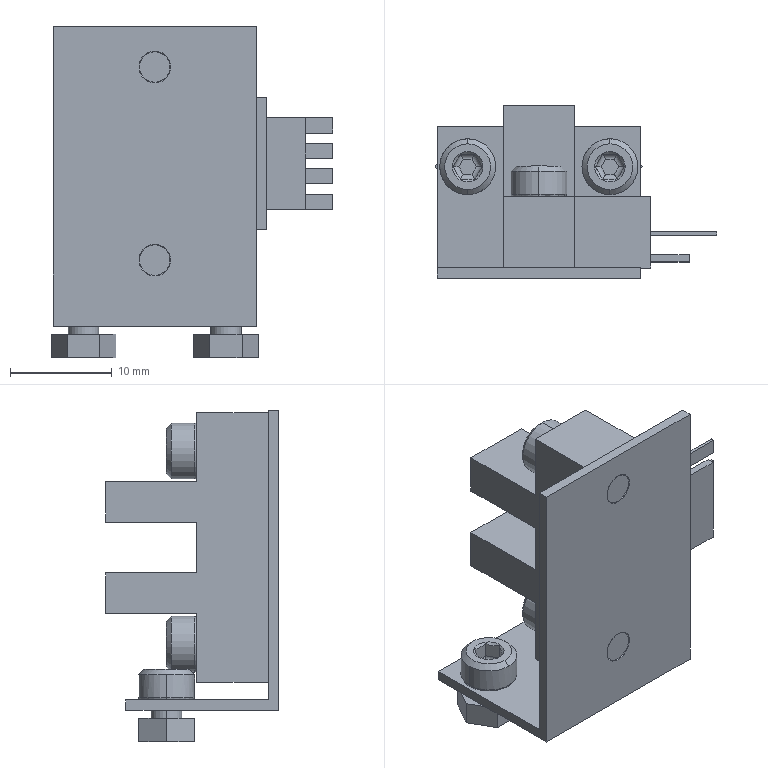Part | SolidWorks | features BaseBody 1 | 1 solid | 189 faces | box 27.675 x 17 x 32.6 mm | volume 3746 mm3 | plane 109 | cylinder 52 | cone 20 | spline 8 | commonest cylinder face diameters 1 x24 3 x16 5.5 x8 3.2 x4